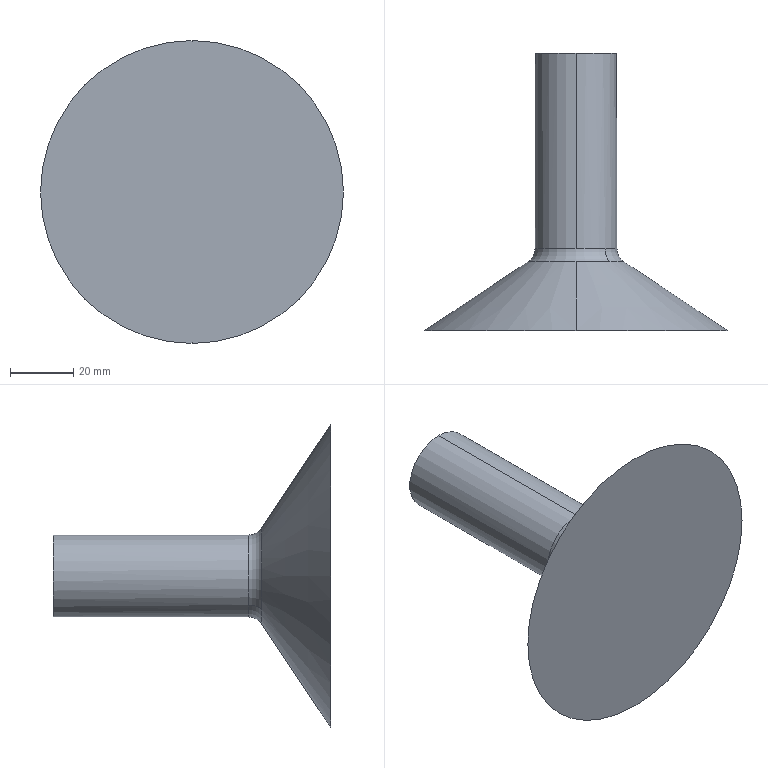Part | STEP file | ASND-0110-1.120ww | 1 solid | 14 faces | box 96.056 x 88 x 96.056 mm | volume 106190 mm3 | cylinder 4 | cone 4 | plane 4 | torus 2 | commonest cylinder face diameters 6 x2 26 x2
STEP:
#1=CARTESIAN_POINT('',(0.,0.,0.));
#2=DIRECTION('',(0.,0.,1.));
#3=DIRECTION('',(1.,0.,0.));
#4=AXIS2_PLACEMENT_3D('',#1,#2,#3);
#5=CARTESIAN_POINT('',(0.,11.868,-15.226));
#6=VERTEX_POINT('',#5);
#7=CARTESIAN_POINT('',(10.767,11.868,10.767));
#8=VERTEX_POINT('',#7);
#9=CARTESIAN_POINT('',(0.,11.868,0.));
#10=DIRECTION('',(0.,-1.,0.));
#11=DIRECTION('',(0.,0.,-1.));
#12=AXIS2_PLACEMENT_3D('',#9,#10,#11);
#13=CIRCLE('',#12,15.226);
#14=CARTESIAN_POINT('',(0.,16.028,0.));
#15=DIRECTION('',(0.,-1.,0.));
#16=DIRECTION('',(0.7071,0.,0.7071));
#17=AXIS2_PLACEMENT_3D('',#14,#15,#16);
#18=TOROIDAL_SURFACE('',#17,18.,5.);
#19=CARTESIAN_POINT('',(3.927,2.159));
#20=DIRECTION('',(1.,0.));
#21=VECTOR('',#20,1.);
#22=LINE('',#19,#21);
#23=(GEOMETRIC_REPRESENTATION_CONTEXT(2)PARAMETRIC_REPRESENTATION_CONTEXT()REPRESENTATION_CONTEXT('',''));
#24=DEFINITIONAL_REPRESENTATION('',(#22),#23);
#25=PCURVE('',#18,#24);
#26=CARTESIAN_POINT('',(0.,-10.,0.));
#27=DIRECTION('',(0.,-1.,0.));
#28=DIRECTION('',(0.,0.,-1.));
#29=AXIS2_PLACEMENT_3D('',#26,#27,#28);
#30=CONICAL_SURFACE('',#29,48.028,0.9828);
#31=CARTESIAN_POINT('',(0.,-21.868));
#32=DIRECTION('',(1.,0.));
#33=VECTOR('',#32,1.);
#34=LINE('',#31,#33);
#35=(GEOMETRIC_REPRESENTATION_CONTEXT(2)PARAMETRIC_REPRESENTATION_CONTEXT()REPRESENTATION_CONTEXT('',''));
#36=DEFINITIONAL_REPRESENTATION('',(#34),#35);
#37=PCURVE('',#30,#36);
#38=SURFACE_CURVE('',#13,(#25,#37),.PCURVE_S1.);
#39=EDGE_CURVE('',#6,#8,#38,.T.);
#40=ORIENTED_EDGE('',*,*,#39,.T.);
#41=CARTESIAN_POINT('',(9.192,16.028,9.192));
#42=VERTEX_POINT('',#41);
#43=CARTESIAN_POINT('',(12.728,16.028,12.728));
#44=DIRECTION('',(0.7071,0.,-0.7071));
#45=DIRECTION('',(-0.7071,0.,-0.7071));
#46=AXIS2_PLACEMENT_3D('',#43,#44,#45);
#47=CIRCLE('',#46,5.);
#48=CARTESIAN_POINT('',(6.283,-3.142));
#49=DIRECTION('',(0.,1.));
#50=VECTOR('',#49,1.);
#51=LINE('',#48,#50);
#52=(GEOMETRIC_REPRESENTATION_CONTEXT(2)PARAMETRIC_REPRESENTATION_CONTEXT()REPRESENTATION_CONTEXT('',''));
#53=DEFINITIONAL_REPRESENTATION('',(#51),#52);
#54=PCURVE('',#18,#53);
#55=CARTESIAN_POINT('',(0.,16.028,0.));
#56=DIRECTION('',(0.,-1.,0.));
#57=DIRECTION('',(0.7071,0.,0.7071));
#58=AXIS2_PLACEMENT_3D('',#55,#56,#57);
#59=TOROIDAL_SURFACE('',#58,18.,5.);
#60=CARTESIAN_POINT('',(0.,-3.142));
#61=DIRECTION('',(0.,1.));
#62=VECTOR('',#61,1.);
#63=LINE('',#60,#62);
#64=(GEOMETRIC_REPRESENTATION_CONTEXT(2)PARAMETRIC_REPRESENTATION_CONTEXT()REPRESENTATION_CONTEXT('',''));
#65=DEFINITIONAL_REPRESENTATION('',(#63),#64);
#66=PCURVE('',#59,#65);
#67=SURFACE_CURVE('',#47,(#54,#66),.PCURVE_S1.);
#68=EDGE_CURVE('',#8,#42,#67,.T.);
#69=ORIENTED_EDGE('',*,*,#68,.T.);
#70=CARTESIAN_POINT('',(0.,16.028,-13.));
#71=VERTEX_POINT('',#70);
#72=CARTESIAN_POINT('',(0.,16.028,0.));
#73=DIRECTION('',(0.,1.,0.));
#74=DIRECTION('',(0.,0.,-1.));
#75=AXIS2_PLACEMENT_3D('',#72,#73,#74);
#76=CIRCLE('',#75,13.);
#77=CARTESIAN_POINT('',(10.21,3.142));
#78=DIRECTION('',(-1.,0.));
#79=VECTOR('',#78,1.);
#80=LINE('',#77,#79);
#81=(GEOMETRIC_REPRESENTATION_CONTEXT(2)PARAMETRIC_REPRESENTATION_CONTEXT()REPRESENTATION_CONTEXT('',''));
#82=DEFINITIONAL_REPRESENTATION('',(#80),#81);
#83=PCURVE('',#18,#82);
#84=CARTESIAN_POINT('',(0.,0.,0.));
#85=DIRECTION('',(0.,-1.,0.));
#86=DIRECTION('',(0.,0.,-1.));
#87=AXIS2_PLACEMENT_3D('',#84,#85,#86);
#88=CYLINDRICAL_SURFACE('',#87,13.);
#89=CARTESIAN_POINT('',(6.283,-16.028));
#90=DIRECTION('',(-1.,0.));
#91=VECTOR('',#90,1.);
#92=LINE('',#89,#91);
#93=(GEOMETRIC_REPRESENTATION_CONTEXT(2)PARAMETRIC_REPRESENTATION_CONTEXT()REPRESENTATION_CONTEXT('',''));
#94=DEFINITIONAL_REPRESENTATION('',(#92),#93);
#95=PCURVE('',#88,#94);
#96=SURFACE_CURVE('',#76,(#83,#95),.PCURVE_S1.);
#97=EDGE_CURVE('',#42,#71,#96,.T.);
#98=ORIENTED_EDGE('',*,*,#97,.T.);
#99=CARTESIAN_POINT('',(-9.192,16.028,-9.192));
#100=VERTEX_POINT('',#99);
#101=CARTESIAN_POINT('',(0.,16.028,0.));
#102=DIRECTION('',(0.,1.,0.));
#103=DIRECTION('',(0.,0.,-1.));
#104=AXIS2_PLACEMENT_3D('',#101,#102,#103);
#105=CIRCLE('',#104,13.);
#106=CARTESIAN_POINT('',(3.927,3.142));
#107=DIRECTION('',(-1.,0.));
#108=VECTOR('',#107,1.);
#109=LINE('',#106,#108);
#110=(GEOMETRIC_REPRESENTATION_CONTEXT(2)PARAMETRIC_REPRESENTATION_CONTEXT()REPRESENTATION_CONTEXT('',''));
#111=DEFINITIONAL_REPRESENTATION('',(#109),#110);
#112=PCURVE('',#18,#111);
#113=CARTESIAN_POINT('',(0.,0.,0.));
#114=DIRECTION('',(0.,-1.,0.));
#115=DIRECTION('',(0.,0.,-1.));
#116=AXIS2_PLACEMENT_3D('',#113,#114,#115);
#117=CYLINDRICAL_SURFACE('',#116,13.);
#118=CARTESIAN_POINT('',(6.283,-16.028));
#119=DIRECTION('',(-1.,0.));
#120=VECTOR('',#119,1.);
#121=LINE('',#118,#120);
#122=(GEOMETRIC_REPRESENTATION_CONTEXT(2)PARAMETRIC_REPRESENTATION_CONTEXT()REPRESENTATION_CONTEXT('',''));
#123=DEFINITIONAL_REPRESENTATION('',(#121),#122);
#124=PCURVE('',#117,#123);
#125=SURFACE_CURVE('',#105,(#112,#124),.PCURVE_S1.);
#126=EDGE_CURVE('',#71,#100,#125,.T.);
#127=ORIENTED_EDGE('',*,*,#126,.T.);
#128=CARTESIAN_POINT('',(-10.767,11.868,-10.767));
#129=VERTEX_POINT('',#128);
#130=CARTESIAN_POINT('',(-12.728,16.028,-12.728));
#131=DIRECTION('',(-0.7071,0.,0.7071));
#132=DIRECTION('',(0.7071,0.,0.7071));
#133=AXIS2_PLACEMENT_3D('',#130,#131,#132);
#134=CIRCLE('',#133,5.);
#135=CARTESIAN_POINT('',(3.142,-3.142));
#136=DIRECTION('',(0.,1.));
#137=VECTOR('',#136,1.);
#138=LINE('',#135,#137);
#139=(GEOMETRIC_REPRESENTATION_CONTEXT(2)PARAMETRIC_REPRESENTATION_CONTEXT()REPRESENTATION_CONTEXT('',''));
#140=DEFINITIONAL_REPRESENTATION('',(#138),#139);
#141=PCURVE('',#18,#140);
#142=CARTESIAN_POINT('',(3.142,-3.142));
#143=DIRECTION('',(0.,1.));
#144=VECTOR('',#143,1.);
#145=LINE('',#142,#144);
#146=(GEOMETRIC_REPRESENTATION_CONTEXT(2)PARAMETRIC_REPRESENTATION_CONTEXT()REPRESENTATION_CONTEXT('',''));
#147=DEFINITIONAL_REPRESENTATION('',(#145),#146);
#148=PCURVE('',#59,#147);
#149=SURFACE_CURVE('',#134,(#141,#148),.PCURVE_S1.);
#150=EDGE_CURVE('',#129,#100,#149,.T.);
#151=ORIENTED_EDGE('',*,*,#150,.F.);
#152=CARTESIAN_POINT('',(0.,11.868,0.));
#153=DIRECTION('',(0.,-1.,0.));
#154=DIRECTION('',(0.,0.,-1.));
#155=AXIS2_PLACEMENT_3D('',#152,#153,#154);
#156=CIRCLE('',#155,15.226);
#157=CARTESIAN_POINT('',(-2.356,2.159));
#158=DIRECTION('',(1.,0.));
#159=VECTOR('',#158,1.);
#160=LINE('',#157,#159);
#161=(GEOMETRIC_REPRESENTATION_CONTEXT(2)PARAMETRIC_REPRESENTATION_CONTEXT()REPRESENTATION_CONTEXT('',''));
#162=DEFINITIONAL_REPRESENTATION('',(#160),#161);
#163=PCURVE('',#18,#162);
#164=CARTESIAN_POINT('',(0.,-10.,0.));
#165=DIRECTION('',(0.,-1.,0.));
#166=DIRECTION('',(0.,0.,-1.));
#167=AXIS2_PLACEMENT_3D('',#164,#165,#166);
#168=CONICAL_SURFACE('',#167,48.028,0.9828);
#169=CARTESIAN_POINT('',(0.,-21.868));
#170=DIRECTION('',(1.,0.));
#171=VECTOR('',#170,1.);
#172=LINE('',#169,#171);
#173=(GEOMETRIC_REPRESENTATION_CONTEXT(2)PARAMETRIC_REPRESENTATION_CONTEXT()REPRESENTATION_CONTEXT('',''));
#174=DEFINITIONAL_REPRESENTATION('',(#172),#173);
#175=PCURVE('',#168,#174);
#176=SURFACE_CURVE('',#156,(#163,#175),.PCURVE_S1.);
#177=EDGE_CURVE('',#129,#6,#176,.T.);
#178=ORIENTED_EDGE('',*,*,#177,.T.);
#179=EDGE_LOOP('',(#40,#69,#98,#127,#151,#178));
#180=FACE_BOUND('',#179,.F.);
#181=ADVANCED_FACE('',(#180),#18,.F.);
#182=CARTESIAN_POINT('',(0.,78.,-13.));
#183=VERTEX_POINT('',#182);
#184=CARTESIAN_POINT('',(0.,78.,13.));
#185=VERTEX_POINT('',#184);
#186=CARTESIAN_POINT('',(0.,78.,0.));
#187=DIRECTION('',(0.,-1.,0.));
#188=DIRECTION('',(0.,0.,-1.));
#189=AXIS2_PLACEMENT_3D('',#186,#187,#188);
#190=CIRCLE('',#189,13.);
#191=CARTESIAN_POINT('',(0.,-78.));
#192=DIRECTION('',(1.,0.));
#193=VECTOR('',#192,1.);
#194=LINE('',#191,#193);
#195=(GEOMETRIC_REPRESENTATION_CONTEXT(2)PARAMETRIC_REPRESENTATION_CONTEXT()REPRESENTATION_CONTEXT('',''));
#196=DEFINITIONAL_REPRESENTATION('',(#194),#195);
#197=PCURVE('',#88,#196);
#198=CARTESIAN_POINT('',(3.,78.,0.));
#199=DIRECTION('',(0.,1.,0.));
#200=DIRECTION('',(0.7071,0.,0.7071));
#201=AXIS2_PLACEMENT_3D('',#198,#199,#200);
#202=PLANE('',#201);
#203=CARTESIAN_POINT('',(-11.314,7.071));
#204=CARTESIAN_POINT('',(4.608,22.993));
#205=CARTESIAN_POINT('',(10.436,1.243));
#206=CARTESIAN_POINT('',(16.263,-20.506));
#207=CARTESIAN_POINT('',(-5.486,-14.678));
#208=CARTESIAN_POINT('',(-27.235,-8.851));
#209=CARTESIAN_POINT('',(-11.314,7.071));
#210=(BOUNDED_CURVE()B_SPLINE_CURVE(2,(#203,#204,#205,#206,#207,#208,#209),.UNSPECIFIED.,.T.,.F.)B_SPLINE_CURVE_WITH_KNOTS((1,2,2,2,2,1),(-2.094,0.,2.094,4.189,6.283,8.378),.UNSPECIFIED.)CURVE()GEOMETRIC_REPRESENTATION_ITEM()RATIONAL_B_SPLINE_CURVE((1.,0.5,1.,0.5,1.,0.5,1.))REPRESENTATION_ITEM(''));
#211=(GEOMETRIC_REPRESENTATION_CONTEXT(2)PARAMETRIC_REPRESENTATION_CONTEXT()REPRESENTATION_CONTEXT('',''));
#212=DEFINITIONAL_REPRESENTATION('',(#210),#211);
#213=PCURVE('',#202,#212);
#214=SURFACE_CURVE('',#190,(#197,#213),.PCURVE_S1.);
#215=EDGE_CURVE('',#183,#185,#214,.T.);
#216=ORIENTED_EDGE('',*,*,#215,.T.);
#217=CARTESIAN_POINT('',(0.,16.028,13.));
#218=VERTEX_POINT('',#217);
#219=CARTESIAN_POINT('',(0.,0.,13.));
#220=DIRECTION('',(0.,-1.,0.));
#221=VECTOR('',#220,1.);
#222=LINE('',#219,#221);
#223=CARTESIAN_POINT('',(3.142,0.));
#224=DIRECTION('',(0.,1.));
#225=VECTOR('',#224,1.);
#226=LINE('',#223,#225);
#227=(GEOMETRIC_REPRESENTATION_CONTEXT(2)PARAMETRIC_REPRESENTATION_CONTEXT()REPRESENTATION_CONTEXT('',''));
#228=DEFINITIONAL_REPRESENTATION('',(#226),#227);
#229=PCURVE('',#88,#228);
#230=CARTESIAN_POINT('',(3.142,0.));
#231=DIRECTION('',(0.,1.));
#232=VECTOR('',#231,1.);
#233=LINE('',#230,#232);
#234=(GEOMETRIC_REPRESENTATION_CONTEXT(2)PARAMETRIC_REPRESENTATION_CONTEXT()REPRESENTATION_CONTEXT('',''));
#235=DEFINITIONAL_REPRESENTATION('',(#233),#234);
#236=PCURVE('',#117,#235);
#237=SURFACE_CURVE('',#222,(#229,#236),.PCURVE_S1.);
#238=EDGE_CURVE('',#185,#218,#237,.T.);
#239=ORIENTED_EDGE('',*,*,#238,.T.);
#240=CARTESIAN_POINT('',(0.,16.028,0.));
#241=DIRECTION('',(0.,1.,0.));
#242=DIRECTION('',(0.,0.,-1.));
#243=AXIS2_PLACEMENT_3D('',#240,#241,#242);
#244=CIRCLE('',#243,13.);
#245=CARTESIAN_POINT('',(6.283,-16.028));
#246=DIRECTION('',(-1.,0.));
#247=VECTOR('',#246,1.);
#248=LINE('',#245,#247);
#249=(GEOMETRIC_REPRESENTATION_CONTEXT(2)PARAMETRIC_REPRESENTATION_CONTEXT()REPRESENTATION_CONTEXT('',''));
#250=DEFINITIONAL_REPRESENTATION('',(#248),#249);
#251=PCURVE('',#88,#250);
#252=CARTESIAN_POINT('',(3.927,3.142));
#253=DIRECTION('',(-1.,0.));
#254=VECTOR('',#253,1.);
#255=LINE('',#252,#254);
#256=(GEOMETRIC_REPRESENTATION_CONTEXT(2)PARAMETRIC_REPRESENTATION_CONTEXT()REPRESENTATION_CONTEXT('',''));
#257=DEFINITIONAL_REPRESENTATION('',(#255),#256);
#258=PCURVE('',#59,#257);
#259=SURFACE_CURVE('',#244,(#251,#258),.PCURVE_S1.);
#260=EDGE_CURVE('',#218,#42,#259,.T.);
#261=ORIENTED_EDGE('',*,*,#260,.T.);
#262=ORIENTED_EDGE('',*,*,#97,.T.);
#263=CARTESIAN_POINT('',(0.,0.,-13.));
#264=DIRECTION('',(0.,-1.,0.));
#265=VECTOR('',#264,1.);
#266=LINE('',#263,#265);
#267=CARTESIAN_POINT('',(0.,0.));
#268=DIRECTION('',(0.,1.));
#269=VECTOR('',#268,1.);
#270=LINE('',#267,#269);
#271=(GEOMETRIC_REPRESENTATION_CONTEXT(2)PARAMETRIC_REPRESENTATION_CONTEXT()REPRESENTATION_CONTEXT('',''));
#272=DEFINITIONAL_REPRESENTATION('',(#270),#271);
#273=PCURVE('',#88,#272);
#274=CARTESIAN_POINT('',(6.283,0.));
#275=DIRECTION('',(0.,1.));
#276=VECTOR('',#275,1.);
#277=LINE('',#274,#276);
#278=(GEOMETRIC_REPRESENTATION_CONTEXT(2)PARAMETRIC_REPRESENTATION_CONTEXT()REPRESENTATION_CONTEXT('',''));
#279=DEFINITIONAL_REPRESENTATION('',(#277),#278);
#280=PCURVE('',#117,#279);
#281=SURFACE_CURVE('',#266,(#273,#280),.PCURVE_S1.);
#282=EDGE_CURVE('',#183,#71,#281,.T.);
#283=ORIENTED_EDGE('',*,*,#282,.F.);
#284=EDGE_LOOP('',(#216,#239,#261,#262,#283));
#285=FACE_BOUND('',#284,.T.);
#286=ADVANCED_FACE('',(#285),#88,.T.);
#287=ORIENTED_EDGE('',*,*,#39,.T.);
#288=CARTESIAN_POINT('',(0.,11.868,15.226));
#289=VERTEX_POINT('',#288);
#290=CARTESIAN_POINT('',(0.,11.868,0.));
#291=DIRECTION('',(0.,-1.,0.));
#292=DIRECTION('',(0.,0.,-1.));
#293=AXIS2_PLACEMENT_3D('',#290,#291,#292);
#294=CIRCLE('',#293,15.226);
#295=CARTESIAN_POINT('',(0.,-21.868));
#296=DIRECTION('',(1.,0.));
#297=VECTOR('',#296,1.);
#298=LINE('',#295,#297);
#299=(GEOMETRIC_REPRESENTATION_CONTEXT(2)PARAMETRIC_REPRESENTATION_CONTEXT()REPRESENTATION_CONTEXT('',''));
#300=DEFINITIONAL_REPRESENTATION('',(#298),#299);
#301=PCURVE('',#30,#300);
#302=CARTESIAN_POINT('',(-2.356,2.159));
#303=DIRECTION('',(1.,0.));
#304=VECTOR('',#303,1.);
#305=LINE('',#302,#304);
#306=(GEOMETRIC_REPRESENTATION_CONTEXT(2)PARAMETRIC_REPRESENTATION_CONTEXT()REPRESENTATION_CONTEXT('',''));
#307=DEFINITIONAL_REPRESENTATION('',(#305),#306);
#308=PCURVE('',#59,#307);
#309=SURFACE_CURVE('',#294,(#301,#308),.PCURVE_S1.);
#310=EDGE_CURVE('',#8,#289,#309,.T.);
#311=ORIENTED_EDGE('',*,*,#310,.T.);
#312=CARTESIAN_POINT('',(0.,-10.,48.028));
#313=VERTEX_POINT('',#312);
#314=CARTESIAN_POINT('',(0.,-10.,48.028));
#315=DIRECTION('',(0.,-0.5547,0.8321));
#316=VECTOR('',#315,1.);
#317=LINE('',#314,#316);
#318=CARTESIAN_POINT('',(3.142,0.));
#319=DIRECTION('',(0.,1.));
#320=VECTOR('',#319,1.);
#321=LINE('',#318,#320);
#322=(GEOMETRIC_REPRESENTATION_CONTEXT(2)PARAMETRIC_REPRESENTATION_CONTEXT()REPRESENTATION_CONTEXT('',''));
#323=DEFINITIONAL_REPRESENTATION('',(#321),#322);
#324=PCURVE('',#30,#323);
#325=CARTESIAN_POINT('',(3.142,0.));
#326=DIRECTION('',(0.,1.));
#327=VECTOR('',#326,1.);
#328=LINE('',#325,#327);
#329=(GEOMETRIC_REPRESENTATION_CONTEXT(2)PARAMETRIC_REPRESENTATION_CONTEXT()REPRESENTATION_CONTEXT('',''));
#330=DEFINITIONAL_REPRESENTATION('',(#328),#329);
#331=PCURVE('',#168,#330);
#332=SURFACE_CURVE('',#317,(#324,#331),.PCURVE_S1.);
#333=EDGE_CURVE('',#289,#313,#332,.T.);
#334=ORIENTED_EDGE('',*,*,#333,.T.);
#335=CARTESIAN_POINT('',(0.,-10.,-48.028));
#336=VERTEX_POINT('',#335);
#337=CARTESIAN_POINT('',(0.,-10.,0.));
#338=DIRECTION('',(0.,-1.,0.));
#339=DIRECTION('',(0.,0.,-1.));
#340=AXIS2_PLACEMENT_3D('',#337,#338,#339);
#341=CIRCLE('',#340,48.028);
#342=CARTESIAN_POINT('',(0.,0.));
#343=DIRECTION('',(1.,0.));
#344=VECTOR('',#343,1.);
#345=LINE('',#342,#344);
#346=(GEOMETRIC_REPRESENTATION_CONTEXT(2)PARAMETRIC_REPRESENTATION_CONTEXT()REPRESENTATION_CONTEXT('',''));
#347=DEFINITIONAL_REPRESENTATION('',(#345),#346);
#348=PCURVE('',#30,#347);
#349=CARTESIAN_POINT('',(0.,-10.,0.));
#350=DIRECTION('',(0.,-1.,0.));
#351=DIRECTION('',(0.7071,0.,0.7071));
#352=AXIS2_PLACEMENT_3D('',#349,#350,#351);
#353=PLANE('',#352);
#354=CARTESIAN_POINT('',(0.,0.));
#355=DIRECTION('',(-0.7071,-0.7071));
#356=AXIS2_PLACEMENT_2D('',#354,#355);
#357=CIRCLE('',#356,48.028);
#358=(GEOMETRIC_REPRESENTATION_CONTEXT(2)PARAMETRIC_REPRESENTATION_CONTEXT()REPRESENTATION_CONTEXT('',''));
#359=DEFINITIONAL_REPRESENTATION('',(#357),#358);
#360=PCURVE('',#353,#359);
#361=SURFACE_CURVE('',#341,(#348,#360),.PCURVE_S1.);
#362=EDGE_CURVE('',#336,#313,#361,.T.);
#363=ORIENTED_EDGE('',*,*,#362,.F.);
#364=CARTESIAN_POINT('',(0.,-10.,-48.028));
#365=DIRECTION('',(0.,-0.5547,-0.8321));
#366=VECTOR('',#365,1.);
#367=LINE('',#364,#366);
#368=CARTESIAN_POINT('',(0.,0.));
#369=DIRECTION('',(0.,1.));
#370=VECTOR('',#369,1.);
#371=LINE('',#368,#370);
#372=(GEOMETRIC_REPRESENTATION_CONTEXT(2)PARAMETRIC_REPRESENTATION_CONTEXT()REPRESENTATION_CONTEXT('',''));
#373=DEFINITIONAL_REPRESENTATION('',(#371),#372);
#374=PCURVE('',#30,#373);
#375=CARTESIAN_POINT('',(6.283,0.));
#376=DIRECTION('',(0.,1.));
#377=VECTOR('',#376,1.);
#378=LINE('',#375,#377);
#379=(GEOMETRIC_REPRESENTATION_CONTEXT(2)PARAMETRIC_REPRESENTATION_CONTEXT()REPRESENTATION_CONTEXT('',''));
#380=DEFINITIONAL_REPRESENTATION('',(#378),#379);
#381=PCURVE('',#168,#380);
#382=SURFACE_CURVE('',#367,(#374,#381),.PCURVE_S1.);
#383=EDGE_CURVE('',#6,#336,#382,.T.);
#384=ORIENTED_EDGE('',*,*,#383,.F.);
#385=EDGE_LOOP('',(#287,#311,#334,#363,#384));
#386=FACE_BOUND('',#385,.T.);
#387=ADVANCED_FACE('',(#386),#30,.T.);
#388=ORIENTED_EDGE('',*,*,#215,.F.);
#389=CARTESIAN_POINT('',(0.,78.,0.));
#390=DIRECTION('',(0.,-1.,0.));
#391=DIRECTION('',(0.,0.,-1.));
#392=AXIS2_PLACEMENT_3D('',#389,#390,#391);
#393=CIRCLE('',#392,13.);
#394=CARTESIAN_POINT('',(-11.314,7.071));
#395=CARTESIAN_POINT('',(4.608,22.993));
#396=CARTESIAN_POINT('',(10.436,1.243));
#397=CARTESIAN_POINT('',(16.263,-20.506));
#398=CARTESIAN_POINT('',(-5.486,-14.678));
#399=CARTESIAN_POINT('',(-27.235,-8.851));
#400=CARTESIAN_POINT('',(-11.314,7.071));
#401=(BOUNDED_CURVE()B_SPLINE_CURVE(2,(#394,#395,#396,#397,#398,#399,#400),.UNSPECIFIED.,.T.,.F.)B_SPLINE_CURVE_WITH_KNOTS((1,2,2,2,2,1),(-2.094,0.,2.094,4.189,6.283,8.378),.UNSPECIFIED.)CURVE()GEOMETRIC_REPRESENTATION_ITEM()RATIONAL_B_SPLINE_CURVE((1.,0.5,1.,0.5,1.,0.5,1.))REPRESENTATION_ITEM(''));
#402=(GEOMETRIC_REPRESENTATION_CONTEXT(2)PARAMETRIC_REPRESENTATION_CONTEXT()REPRESENTATION_CONTEXT('',''));
#403=DEFINITIONAL_REPRESENTATION('',(#401),#402);
#404=PCURVE('',#202,#403);
#405=CARTESIAN_POINT('',(0.,-78.));
#406=DIRECTION('',(1.,0.));
#407=VECTOR('',#406,1.);
#408=LINE('',#405,#407);
#409=(GEOMETRIC_REPRESENTATION_CONTEXT(2)PARAMETRIC_REPRESENTATION_CONTEXT()REPRESENTATION_CONTEXT('',''));
#410=DEFINITIONAL_REPRESENTATION('',(#408),#409);
#411=PCURVE('',#117,#410);
#412=SURFACE_CURVE('',#393,(#404,#411),.PCURVE_S1.);
#413=EDGE_CURVE('',#185,#183,#412,.T.);
#414=ORIENTED_EDGE('',*,*,#413,.F.);
#415=EDGE_LOOP('',(#388,#414));
#416=FACE_BOUND('',#415,.T.);
#417=ADVANCED_FACE('',(#416),#202,.T.);
#418=ORIENTED_EDGE('',*,*,#362,.T.);
#419=CARTESIAN_POINT('',(0.,-10.,0.));
#420=DIRECTION('',(0.,-1.,0.));
#421=DIRECTION('',(0.,0.,-1.));
#422=AXIS2_PLACEMENT_3D('',#419,#420,#421);
#423=CIRCLE('',#422,48.028);
#424=CARTESIAN_POINT('',(0.,0.));
#425=DIRECTION('',(-0.7071,-0.7071));
#426=AXIS2_PLACEMENT_2D('',#424,#425);
#427=CIRCLE('',#426,48.028);
#428=(GEOMETRIC_REPRESENTATION_CONTEXT(2)PARAMETRIC_REPRESENTATION_CONTEXT()REPRESENTATION_CONTEXT('',''));
#429=DEFINITIONAL_REPRESENTATION('',(#427),#428);
#430=PCURVE('',#353,#429);
#431=CARTESIAN_POINT('',(0.,0.));
#432=DIRECTION('',(1.,0.));
#433=VECTOR('',#432,1.);
#434=LINE('',#431,#433);
#435=(GEOMETRIC_REPRESENTATION_CONTEXT(2)PARAMETRIC_REPRESENTATION_CONTEXT()REPRESENTATION_CONTEXT('',''));
#436=DEFINITIONAL_REPRESENTATION('',(#434),#435);
#437=PCURVE('',#168,#436);
#438=SURFACE_CURVE('',#423,(#430,#437),.PCURVE_S1.);
#439=EDGE_CURVE('',#313,#336,#438,.T.);
#440=ORIENTED_EDGE('',*,*,#439,.T.);
#441=EDGE_LOOP('',(#418,#440));
#442=FACE_BOUND('',#441,.T.);
#443=ADVANCED_FACE('',(#442),#353,.T.);
#444=ORIENTED_EDGE('',*,*,#333,.F.);
#445=CARTESIAN_POINT('',(0.,11.868,0.));
#446=DIRECTION('',(0.,-1.,0.));
#447=DIRECTION('',(0.,0.,-1.));
#448=AXIS2_PLACEMENT_3D('',#445,#446,#447);
#449=CIRCLE('',#448,15.226);
#450=CARTESIAN_POINT('',(0.,-21.868));
#451=DIRECTION('',(1.,0.));
#452=VECTOR('',#451,1.);
#453=LINE('',#450,#452);
#454=(GEOMETRIC_REPRESENTATION_CONTEXT(2)PARAMETRIC_REPRESENTATION_CONTEXT()REPRESENTATION_CONTEXT('',''));
#455=DEFINITIONAL_REPRESENTATION('',(#453),#454);
#456=PCURVE('',#168,#455);
#457=CARTESIAN_POINT('',(-2.356,2.159));
#458=DIRECTION('',(1.,0.));
#459=VECTOR('',#458,1.);
#460=LINE('',#457,#459);
#461=(GEOMETRIC_REPRESENTATION_CONTEXT(2)PARAMETRIC_REPRESENTATION_CONTEXT()REPRESENTATION_CONTEXT('',''));
#462=DEFINITIONAL_REPRESENTATION('',(#460),#461);
#463=PCURVE('',#59,#462);
#464=SURFACE_CURVE('',#449,(#456,#463),.PCURVE_S1.);
#465=EDGE_CURVE('',#289,#129,#464,.T.);
#466=ORIENTED_EDGE('',*,*,#465,.T.);
#467=ORIENTED_EDGE('',*,*,#177,.T.);
#468=ORIENTED_EDGE('',*,*,#383,.T.);
#469=ORIENTED_EDGE('',*,*,#439,.F.);
#470=EDGE_LOOP('',(#444,#466,#467,#468,#469));
#471=FACE_BOUND('',#470,.T.);
#472=ADVANCED_FACE('',(#471),#168,.T.);
#473=ORIENTED_EDGE('',*,*,#238,.F.);
#474=ORIENTED_EDGE('',*,*,#413,.T.);
#475=ORIENTED_EDGE('',*,*,#282,.T.);
#476=ORIENTED_EDGE('',*,*,#126,.T.);
#477=CARTESIAN_POINT('',(0.,16.028,0.));
#478=DIRECTION('',(0.,1.,0.));
#479=DIRECTION('',(0.,0.,-1.));
#480=AXIS2_PLACEMENT_3D('',#477,#478,#479);
#481=CIRCLE('',#480,13.);
#482=CARTESIAN_POINT('',(6.283,-16.028));
#483=DIRECTION('',(-1.,0.));
#484=VECTOR('',#483,1.);
#485=LINE('',#482,#484);
#486=(GEOMETRIC_REPRESENTATION_CONTEXT(2)PARAMETRIC_REPRESENTATION_CONTEXT()REPRESENTATION_CONTEXT('',''));
#487=DEFINITIONAL_REPRESENTATION('',(#485),#486);
#488=PCURVE('',#117,#487);
#489=CARTESIAN_POINT('',(3.927,3.142));
#490=DIRECTION('',(-1.,0.));
#491=VECTOR('',#490,1.);
#492=LINE('',#489,#491);
#493=(GEOMETRIC_REPRESENTATION_CONTEXT(2)PARAMETRIC_REPRESENTATION_CONTEXT()REPRESENTATION_CONTEXT('',''));
#494=DEFINITIONAL_REPRESENTATION('',(#492),#493);
#495=PCURVE('',#59,#494);
#496=SURFACE_CURVE('',#481,(#488,#495),.PCURVE_S1.);
#497=EDGE_CURVE('',#100,#218,#496,.T.);
#498=ORIENTED_EDGE('',*,*,#497,.T.);
#499=EDGE_LOOP('',(#473,#474,#475,#476,#498));
#500=FACE_BOUND('',#499,.T.);
#501=ADVANCED_FACE('',(#500),#117,.T.);
#502=ORIENTED_EDGE('',*,*,#497,.T.);
#503=ORIENTED_EDGE('',*,*,#260,.T.);
#504=ORIENTED_EDGE('',*,*,#68,.F.);
#505=ORIENTED_EDGE('',*,*,#310,.T.);
#506=ORIENTED_EDGE('',*,*,#465,.T.);
#507=ORIENTED_EDGE('',*,*,#150,.T.);
#508=EDGE_LOOP('',(#502,#503,#504,#505,#506,#507));
#509=FACE_BOUND('',#508,.F.);
#510=ADVANCED_FACE('',(#509),#59,.F.);
#511=CLOSED_SHELL('',(#181,#286,#387,#417,#443,#472,#501,#510));
#512=CARTESIAN_POINT('',(0.,8.,-3.));
#513=VERTEX_POINT('',#512);
#514=CARTESIAN_POINT('',(0.,0.,-15.));
#515=VERTEX_POINT('',#514);
#516=CARTESIAN_POINT('',(0.,0.,-15.));
#517=DIRECTION('',(0.,-0.5547,-0.8321));
#518=VECTOR('',#517,1.);
#519=LINE('',#516,#518);
#520=CARTESIAN_POINT('',(0.,0.,0.));
#521=DIRECTION('',(0.,-1.,0.));
#522=DIRECTION('',(0.,0.,-1.));
#523=AXIS2_PLACEMENT_3D('',#520,#521,#522);
#524=CONICAL_SURFACE('',#523,15.,0.9828);
#525=CARTESIAN_POINT('',(6.283,0.));
#526=DIRECTION('',(0.,1.));
#527=VECTOR('',#526,1.);
#528=LINE('',#525,#527);
#529=(GEOMETRIC_REPRESENTATION_CONTEXT(2)PARAMETRIC_REPRESENTATION_CONTEXT()REPRESENTATION_CONTEXT('',''));
#530=DEFINITIONAL_REPRESENTATION('',(#528),#529);
#531=PCURVE('',#524,#530);
#532=CARTESIAN_POINT('',(0.,0.,0.));
#533=DIRECTION('',(0.,-1.,0.));
#534=DIRECTION('',(0.,0.,-1.));
#535=AXIS2_PLACEMENT_3D('',#532,#533,#534);
#536=CONICAL_SURFACE('',#535,15.,0.9828);
#537=CARTESIAN_POINT('',(0.,0.));
#538=DIRECTION('',(0.,1.));
#539=VECTOR('',#538,1.);
#540=LINE('',#537,#539);
#541=(GEOMETRIC_REPRESENTATION_CONTEXT(2)PARAMETRIC_REPRESENTATION_CONTEXT()REPRESENTATION_CONTEXT('',''));
#542=DEFINITIONAL_REPRESENTATION('',(#540),#541);
#543=PCURVE('',#536,#542);
#544=SURFACE_CURVE('',#519,(#531,#543),.PCURVE_S1.);
#545=EDGE_CURVE('',#513,#515,#544,.T.);
#546=ORIENTED_EDGE('',*,*,#545,.T.);
#547=CARTESIAN_POINT('',(0.,0.,15.));
#548=VERTEX_POINT('',#547);
#549=CARTESIAN_POINT('',(0.,0.,0.));
#550=DIRECTION('',(0.,-1.,0.));
#551=DIRECTION('',(0.,0.,-1.));
#552=AXIS2_PLACEMENT_3D('',#549,#550,#551);
#553=CIRCLE('',#552,15.);
#554=CARTESIAN_POINT('',(0.,0.));
#555=DIRECTION('',(1.,0.));
#556=VECTOR('',#555,1.);
#557=LINE('',#554,#556);
#558=(GEOMETRIC_REPRESENTATION_CONTEXT(2)PARAMETRIC_REPRESENTATION_CONTEXT()REPRESENTATION_CONTEXT('',''));
#559=DEFINITIONAL_REPRESENTATION('',(#557),#558);
#560=PCURVE('',#524,#559);
#561=CARTESIAN_POINT('',(0.,0.,0.));
#562=DIRECTION('',(0.,-1.,0.));
#563=DIRECTION('',(0.7071,0.,0.7071));
#564=AXIS2_PLACEMENT_3D('',#561,#562,#563);
#565=PLANE('',#564);
#566=CARTESIAN_POINT('',(0.,0.));
#567=DIRECTION('',(-0.7071,-0.7071));
#568=AXIS2_PLACEMENT_2D('',#566,#567);
#569=CIRCLE('',#568,15.);
#570=(GEOMETRIC_REPRESENTATION_CONTEXT(2)PARAMETRIC_REPRESENTATION_CONTEXT()REPRESENTATION_CONTEXT('',''));
#571=DEFINITIONAL_REPRESENTATION('',(#569),#570);
#572=PCURVE('',#565,#571);
#573=SURFACE_CURVE('',#553,(#560,#572),.PCURVE_S1.);
#574=EDGE_CURVE('',#548,#515,#573,.T.);
#575=ORIENTED_EDGE('',*,*,#574,.F.);
#576=CARTESIAN_POINT('',(0.,8.,3.));
#577=VERTEX_POINT('',#576);
#578=CARTESIAN_POINT('',(0.,0.,15.));
#579=DIRECTION('',(0.,-0.5547,0.8321));
#580=VECTOR('',#579,1.);
#581=LINE('',#578,#580);
#582=CARTESIAN_POINT('',(3.142,0.));
#583=DIRECTION('',(0.,1.));
#584=VECTOR('',#583,1.);
#585=LINE('',#582,#584);
#586=(GEOMETRIC_REPRESENTATION_CONTEXT(2)PARAMETRIC_REPRESENTATION_CONTEXT()REPRESENTATION_CONTEXT('',''));
#587=DEFINITIONAL_REPRESENTATION('',(#585),#586);
#588=PCURVE('',#524,#587);
#589=CARTESIAN_POINT('',(3.142,0.));
#590=DIRECTION('',(0.,1.));
#591=VECTOR('',#590,1.);
#592=LINE('',#589,#591);
#593=(GEOMETRIC_REPRESENTATION_CONTEXT(2)PARAMETRIC_REPRESENTATION_CONTEXT()REPRESENTATION_CONTEXT('',''));
#594=DEFINITIONAL_REPRESENTATION('',(#592),#593);
#595=PCURVE('',#536,#594);
#596=SURFACE_CURVE('',#581,(#588,#595),.PCURVE_S1.);
#597=EDGE_CURVE('',#577,#548,#596,.T.);
#598=ORIENTED_EDGE('',*,*,#597,.F.);
#599=CARTESIAN_POINT('',(0.,8.,0.));
#600=DIRECTION('',(0.,-1.,0.));
#601=DIRECTION('',(0.,0.,-1.));
#602=AXIS2_PLACEMENT_3D('',#599,#600,#601);
#603=CIRCLE('',#602,3.);
#604=CARTESIAN_POINT('',(0.,-8.));
#605=DIRECTION('',(1.,0.));
#606=VECTOR('',#605,1.);
#607=LINE('',#604,#606);
#608=(GEOMETRIC_REPRESENTATION_CONTEXT(2)PARAMETRIC_REPRESENTATION_CONTEXT()REPRESENTATION_CONTEXT('',''));
#609=DEFINITIONAL_REPRESENTATION('',(#607),#608);
#610=PCURVE('',#524,#609);
#611=CARTESIAN_POINT('',(0.,0.,0.));
#612=DIRECTION('',(0.,-1.,0.));
#613=DIRECTION('',(0.,0.,-1.));
#614=AXIS2_PLACEMENT_3D('',#611,#612,#613);
#615=CYLINDRICAL_SURFACE('',#614,3.);
#616=CARTESIAN_POINT('',(0.,-8.));
#617=DIRECTION('',(1.,0.));
#618=VECTOR('',#617,1.);
#619=LINE('',#616,#618);
#620=(GEOMETRIC_REPRESENTATION_CONTEXT(2)PARAMETRIC_REPRESENTATION_CONTEXT()REPRESENTATION_CONTEXT('',''));
#621=DEFINITIONAL_REPRESENTATION('',(#619),#620);
#622=PCURVE('',#615,#621);
#623=SURFACE_CURVE('',#603,(#610,#622),.PCURVE_S1.);
#624=EDGE_CURVE('',#577,#513,#623,.T.);
#625=ORIENTED_EDGE('',*,*,#624,.T.);
#626=EDGE_LOOP('',(#546,#575,#598,#625));
#627=FACE_BOUND('',#626,.T.);
#628=ADVANCED_FACE('',(#627),#524,.T.);
#629=CARTESIAN_POINT('',(0.,68.,-3.));
#630=VERTEX_POINT('',#629);
#631=CARTESIAN_POINT('',(0.,0.,-3.));
#632=DIRECTION('',(0.,-1.,0.));
#633=VECTOR('',#632,1.);
#634=LINE('',#631,#633);
#635=CARTESIAN_POINT('',(6.283,0.));
#636=DIRECTION('',(0.,1.));
#637=VECTOR('',#636,1.);
#638=LINE('',#635,#637);
#639=(GEOMETRIC_REPRESENTATION_CONTEXT(2)PARAMETRIC_REPRESENTATION_CONTEXT()REPRESENTATION_CONTEXT('',''));
#640=DEFINITIONAL_REPRESENTATION('',(#638),#639);
#641=PCURVE('',#615,#640);
#642=CARTESIAN_POINT('',(0.,0.,0.));
#643=DIRECTION('',(0.,-1.,0.));
#644=DIRECTION('',(0.,0.,-1.));
#645=AXIS2_PLACEMENT_3D('',#642,#643,#644);
#646=CYLINDRICAL_SURFACE('',#645,3.);
#647=CARTESIAN_POINT('',(0.,0.));
#648=DIRECTION('',(0.,1.));
#649=VECTOR('',#648,1.);
#650=LINE('',#647,#649);
#651=(GEOMETRIC_REPRESENTATION_CONTEXT(2)PARAMETRIC_REPRESENTATION_CONTEXT()REPRESENTATION_CONTEXT('',''));
#652=DEFINITIONAL_REPRESENTATION('',(#650),#651);
#653=PCURVE('',#646,#652);
#654=SURFACE_CURVE('',#634,(#641,#653),.PCURVE_S1.);
#655=EDGE_CURVE('',#630,#513,#654,.T.);
#656=ORIENTED_EDGE('',*,*,#655,.T.);
#657=ORIENTED_EDGE('',*,*,#624,.F.);
#658=CARTESIAN_POINT('',(0.,68.,3.));
#659=VERTEX_POINT('',#658);
#660=CARTESIAN_POINT('',(0.,0.,3.));
#661=DIRECTION('',(0.,-1.,0.));
#662=VECTOR('',#661,1.);
#663=LINE('',#660,#662);
#664=CARTESIAN_POINT('',(3.142,0.));
#665=DIRECTION('',(0.,1.));
#666=VECTOR('',#665,1.);
#667=LINE('',#664,#666);
#668=(GEOMETRIC_REPRESENTATION_CONTEXT(2)PARAMETRIC_REPRESENTATION_CONTEXT()REPRESENTATION_CONTEXT('',''));
#669=DEFINITIONAL_REPRESENTATION('',(#667),#668);
#670=PCURVE('',#615,#669);
#671=CARTESIAN_POINT('',(3.142,0.));
#672=DIRECTION('',(0.,1.));
#673=VECTOR('',#672,1.);
#674=LINE('',#671,#673);
#675=(GEOMETRIC_REPRESENTATION_CONTEXT(2)PARAMETRIC_REPRESENTATION_CONTEXT()REPRESENTATION_CONTEXT('',''));
#676=DEFINITIONAL_REPRESENTATION('',(#674),#675);
#677=PCURVE('',#646,#676);
#678=SURFACE_CURVE('',#663,(#670,#677),.PCURVE_S1.);
#679=EDGE_CURVE('',#659,#577,#678,.T.);
#680=ORIENTED_EDGE('',*,*,#679,.F.);
#681=CARTESIAN_POINT('',(0.,68.,0.));
#682=DIRECTION('',(0.,-1.,0.));
#683=DIRECTION('',(0.,0.,-1.));
#684=AXIS2_PLACEMENT_3D('',#681,#682,#683);
#685=CIRCLE('',#684,3.);
#686=CARTESIAN_POINT('',(0.,-68.));
#687=DIRECTION('',(1.,0.));
#688=VECTOR('',#687,1.);
#689=LINE('',#686,#688);
#690=(GEOMETRIC_REPRESENTATION_CONTEXT(2)PARAMETRIC_REPRESENTATION_CONTEXT()REPRESENTATION_CONTEXT('',''));
#691=DEFINITIONAL_REPRESENTATION('',(#689),#690);
#692=PCURVE('',#615,#691);
#693=CARTESIAN_POINT('',(3.,68.,0.));
#694=DIRECTION('',(0.,1.,0.));
#695=DIRECTION('',(0.7071,0.,0.7071));
#696=AXIS2_PLACEMENT_3D('',#693,#694,#695);
#697=PLANE('',#696);
#698=CARTESIAN_POINT('',(-4.243,0.));
#699=CARTESIAN_POINT('',(-0.5684,3.674));
#700=CARTESIAN_POINT('',(0.7765,-1.345));
#701=CARTESIAN_POINT('',(2.121,-6.364));
#702=CARTESIAN_POINT('',(-2.898,-5.019));
#703=CARTESIAN_POINT('',(-7.917,-3.674));
#704=CARTESIAN_POINT('',(-4.243,0.));
#705=(BOUNDED_CURVE()B_SPLINE_CURVE(2,(#698,#699,#700,#701,#702,#703,#704),.UNSPECIFIED.,.T.,.F.)B_SPLINE_CURVE_WITH_KNOTS((1,2,2,2,2,1),(-2.094,0.,2.094,4.189,6.283,8.378),.UNSPECIFIED.)CURVE()GEOMETRIC_REPRESENTATION_ITEM()RATIONAL_B_SPLINE_CURVE((1.,0.5,1.,0.5,1.,0.5,1.))REPRESENTATION_ITEM(''));
#706=(GEOMETRIC_REPRESENTATION_CONTEXT(2)PARAMETRIC_REPRESENTATION_CONTEXT()REPRESENTATION_CONTEXT('',''));
#707=DEFINITIONAL_REPRESENTATION('',(#705),#706);
#708=PCURVE('',#697,#707);
#709=SURFACE_CURVE('',#685,(#692,#708),.PCURVE_S1.);
#710=EDGE_CURVE('',#659,#630,#709,.T.);
#711=ORIENTED_EDGE('',*,*,#710,.T.);
#712=EDGE_LOOP('',(#656,#657,#680,#711));
#713=FACE_BOUND('',#712,.T.);
#714=ADVANCED_FACE('',(#713),#615,.T.);
#715=CARTESIAN_POINT('',(0.,68.,0.));
#716=DIRECTION('',(0.,-1.,0.));
#717=DIRECTION('',(0.,0.,-1.));
#718=AXIS2_PLACEMENT_3D('',#715,#716,#717);
#719=CIRCLE('',#718,3.);
#720=CARTESIAN_POINT('',(-4.243,0.));
#721=CARTESIAN_POINT('',(-0.5684,3.674));
#722=CARTESIAN_POINT('',(0.7765,-1.345));
#723=CARTESIAN_POINT('',(2.121,-6.364));
#724=CARTESIAN_POINT('',(-2.898,-5.019));
#725=CARTESIAN_POINT('',(-7.917,-3.674));
#726=CARTESIAN_POINT('',(-4.243,0.));
#727=(BOUNDED_CURVE()B_SPLINE_CURVE(2,(#720,#721,#722,#723,#724,#725,#726),.UNSPECIFIED.,.T.,.F.)B_SPLINE_CURVE_WITH_KNOTS((1,2,2,2,2,1),(-2.094,0.,2.094,4.189,6.283,8.378),.UNSPECIFIED.)CURVE()GEOMETRIC_REPRESENTATION_ITEM()RATIONAL_B_SPLINE_CURVE((1.,0.5,1.,0.5,1.,0.5,1.))REPRESENTATION_ITEM(''));
#728=(GEOMETRIC_REPRESENTATION_CONTEXT(2)PARAMETRIC_REPRESENTATION_CONTEXT()REPRESENTATION_CONTEXT('',''));
#729=DEFINITIONAL_REPRESENTATION('',(#727),#728);
#730=PCURVE('',#697,#729);
#731=CARTESIAN_POINT('',(0.,-68.));
#732=DIRECTION('',(1.,0.));
#733=VECTOR('',#732,1.);
#734=LINE('',#731,#733);
#735=(GEOMETRIC_REPRESENTATION_CONTEXT(2)PARAMETRIC_REPRESENTATION_CONTEXT()REPRESENTATION_CONTEXT('',''));
#736=DEFINITIONAL_REPRESENTATION('',(#734),#735);
#737=PCURVE('',#646,#736);
#738=SURFACE_CURVE('',#719,(#730,#737),.PCURVE_S1.);
#739=EDGE_CURVE('',#630,#659,#738,.T.);
#740=ORIENTED_EDGE('',*,*,#739,.T.);
#741=ORIENTED_EDGE('',*,*,#710,.T.);
#742=EDGE_LOOP('',(#740,#741));
#743=FACE_BOUND('',#742,.F.);
#744=ADVANCED_FACE('',(#743),#697,.T.);
#745=CARTESIAN_POINT('',(0.,8.,0.));
#746=DIRECTION('',(0.,-1.,0.));
#747=DIRECTION('',(0.,0.,-1.));
#748=AXIS2_PLACEMENT_3D('',#745,#746,#747);
#749=CIRCLE('',#748,3.);
#750=CARTESIAN_POINT('',(0.,-8.));
#751=DIRECTION('',(1.,0.));
#752=VECTOR('',#751,1.);
#753=LINE('',#750,#752);
#754=(GEOMETRIC_REPRESENTATION_CONTEXT(2)PARAMETRIC_REPRESENTATION_CONTEXT()REPRESENTATION_CONTEXT('',''));
#755=DEFINITIONAL_REPRESENTATION('',(#753),#754);
#756=PCURVE('',#646,#755);
#757=CARTESIAN_POINT('',(0.,-8.));
#758=DIRECTION('',(1.,0.));
#759=VECTOR('',#758,1.);
#760=LINE('',#757,#759);
#761=(GEOMETRIC_REPRESENTATION_CONTEXT(2)PARAMETRIC_REPRESENTATION_CONTEXT()REPRESENTATION_CONTEXT('',''));
#762=DEFINITIONAL_REPRESENTATION('',(#760),#761);
#763=PCURVE('',#536,#762);
#764=SURFACE_CURVE('',#749,(#756,#763),.PCURVE_S1.);
#765=EDGE_CURVE('',#513,#577,#764,.T.);
#766=ORIENTED_EDGE('',*,*,#765,.F.);
#767=ORIENTED_EDGE('',*,*,#655,.F.);
#768=ORIENTED_EDGE('',*,*,#739,.T.);
#769=ORIENTED_EDGE('',*,*,#679,.T.);
#770=EDGE_LOOP('',(#766,#767,#768,#769));
#771=FACE_BOUND('',#770,.T.);
#772=ADVANCED_FACE('',(#771),#646,.T.);
#773=CARTESIAN_POINT('',(0.,0.,0.));
#774=DIRECTION('',(0.,-1.,0.));
#775=DIRECTION('',(0.,0.,-1.));
#776=AXIS2_PLACEMENT_3D('',#773,#774,#775);
#777=CIRCLE('',#776,15.);
#778=CARTESIAN_POINT('',(0.,0.));
#779=DIRECTION('',(1.,0.));
#780=VECTOR('',#779,1.);
#781=LINE('',#778,#780);
#782=(GEOMETRIC_REPRESENTATION_CONTEXT(2)PARAMETRIC_REPRESENTATION_CONTEXT()REPRESENTATION_CONTEXT('',''));
#783=DEFINITIONAL_REPRESENTATION('',(#781),#782);
#784=PCURVE('',#536,#783);
#785=CARTESIAN_POINT('',(0.,0.));
#786=DIRECTION('',(-0.7071,-0.7071));
#787=AXIS2_PLACEMENT_2D('',#785,#786);
#788=CIRCLE('',#787,15.);
#789=(GEOMETRIC_REPRESENTATION_CONTEXT(2)PARAMETRIC_REPRESENTATION_CONTEXT()REPRESENTATION_CONTEXT('',''));
#790=DEFINITIONAL_REPRESENTATION('',(#788),#789);
#791=PCURVE('',#565,#790);
#792=SURFACE_CURVE('',#777,(#784,#791),.PCURVE_S1.);
#793=EDGE_CURVE('',#515,#548,#792,.T.);
#794=ORIENTED_EDGE('',*,*,#793,.F.);
#795=ORIENTED_EDGE('',*,*,#545,.F.);
#796=ORIENTED_EDGE('',*,*,#765,.T.);
#797=ORIENTED_EDGE('',*,*,#597,.T.);
#798=EDGE_LOOP('',(#794,#795,#796,#797));
#799=FACE_BOUND('',#798,.T.);
#800=ADVANCED_FACE('',(#799),#536,.T.);
#801=ORIENTED_EDGE('',*,*,#793,.F.);
#802=ORIENTED_EDGE('',*,*,#574,.F.);
#803=EDGE_LOOP('',(#801,#802));
#804=FACE_BOUND('',#803,.F.);
#805=ADVANCED_FACE('',(#804),#565,.T.);
#806=CLOSED_SHELL('',(#628,#714,#744,#772,#800,#805));
#807=ORIENTED_CLOSED_SHELL('',*,#806,.F.);
#808=BREP_WITH_VOIDS('',#511,(#807));
#809=(LENGTH_UNIT()NAMED_UNIT(*)SI_UNIT(.MILLI.,.METRE.));
#810=UNCERTAINTY_MEASURE_WITH_UNIT(LENGTH_MEASURE(0.0000001),#809,'','');
#811=(NAMED_UNIT(*)PLANE_ANGLE_UNIT()SI_UNIT($,.RADIAN.));
#812=(NAMED_UNIT(*)SI_UNIT($,.STERADIAN.)SOLID_ANGLE_UNIT());
#813=(GEOMETRIC_REPRESENTATION_CONTEXT(3)GLOBAL_UNCERTAINTY_ASSIGNED_CONTEXT((#810))GLOBAL_UNIT_ASSIGNED_CONTEXT((#809,#811,#812))REPRESENTATION_CONTEXT('',''));
#814=ADVANCED_BREP_SHAPE_REPRESENTATION('',(#4,#808),#813);